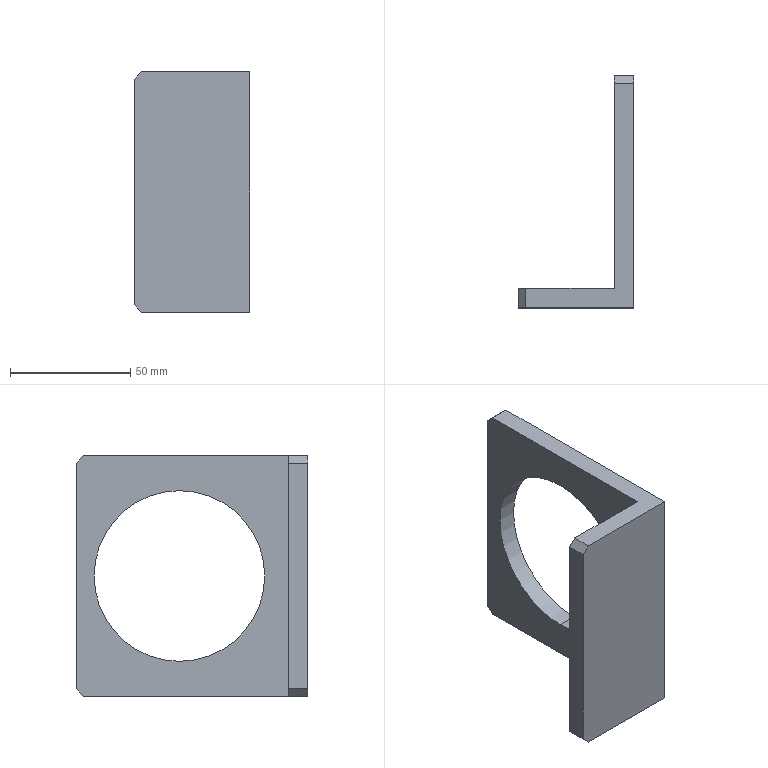Part | SolidWorks | features Chamfer 1, Extrusion 1, ICE 1 | 1 solid | 14 faces | box 48 x 96.5 x 100 mm | volume 77382 mm3 | plane 12 | cylinder 2 | commonest cylinder face diameters 71 x2
STEP:
#1=CARTESIAN_POINT('',(0.,53.5,1.121));
#2=VERTEX_POINT('',#1);
#3=CARTESIAN_POINT('',(0.,53.5,-69.879));
#4=VERTEX_POINT('',#3);
#5=CARTESIAN_POINT('',(0.,53.5,-34.379));
#6=DIRECTION('',(1.,0.,0.));
#7=DIRECTION('',(0.,0.,1.));
#8=AXIS2_PLACEMENT_3D('',#5,#6,#7);
#9=CIRCLE('',#8,35.5);
#10=EDGE_CURVE('',#2,#4,#9,.T.);
#11=ORIENTED_EDGE('',*,*,#10,.T.);
#12=CARTESIAN_POINT('',(-8.,53.5,-69.879));
#13=VERTEX_POINT('',#12);
#14=CARTESIAN_POINT('',(0.001,53.5,-69.879));
#15=DIRECTION('',(-1.,0.,0.));
#16=VECTOR('',#15,1000.);
#17=LINE('',#14,#16);
#18=EDGE_CURVE('',#4,#13,#17,.T.);
#19=ORIENTED_EDGE('',*,*,#18,.T.);
#20=CARTESIAN_POINT('',(-8.,53.5,1.121));
#21=VERTEX_POINT('',#20);
#22=CARTESIAN_POINT('',(-8.,53.5,-34.379));
#23=DIRECTION('',(-1.,0.,0.));
#24=DIRECTION('',(0.,0.,1.));
#25=AXIS2_PLACEMENT_3D('',#22,#23,#24);
#26=CIRCLE('',#25,35.5);
#27=EDGE_CURVE('',#13,#21,#26,.T.);
#28=ORIENTED_EDGE('',*,*,#27,.T.);
#29=CARTESIAN_POINT('',(0.001,53.5,1.121));
#30=DIRECTION('',(-1.,0.,0.));
#31=VECTOR('',#30,1000.);
#32=LINE('',#29,#31);
#33=EDGE_CURVE('',#2,#21,#32,.T.);
#34=ORIENTED_EDGE('',*,*,#33,.F.);
#35=EDGE_LOOP('',(#11,#19,#28,#34));
#36=FACE_OUTER_BOUND('',#35,.T.);
#37=CARTESIAN_POINT('',(0.001,53.5,-34.379));
#38=DIRECTION('',(-1.,0.,0.));
#39=DIRECTION('',(0.,0.,1.));
#40=AXIS2_PLACEMENT_3D('',#37,#38,#39);
#41=CYLINDRICAL_SURFACE('',#40,35.5);
#42=ADVANCED_FACE('',(#36),#41,.F.);
#43=CARTESIAN_POINT('',(-8.,96.5,12.621));
#44=VERTEX_POINT('',#43);
#45=CARTESIAN_POINT('',(-8.,96.5,-81.379));
#46=VERTEX_POINT('',#45);
#47=CARTESIAN_POINT('',(-8.,96.5,15.621));
#48=DIRECTION('',(0.,0.,-1.));
#49=VECTOR('',#48,1000.);
#50=LINE('',#47,#49);
#51=EDGE_CURVE('',#44,#46,#50,.T.);
#52=ORIENTED_EDGE('',*,*,#51,.F.);
#53=CARTESIAN_POINT('',(0.,96.5,12.621));
#54=VERTEX_POINT('',#53);
#55=CARTESIAN_POINT('',(-8.,96.5,12.621));
#56=DIRECTION('',(1.,0.,0.));
#57=VECTOR('',#56,1000.);
#58=LINE('',#55,#57);
#59=EDGE_CURVE('',#44,#54,#58,.T.);
#60=ORIENTED_EDGE('',*,*,#59,.T.);
#61=CARTESIAN_POINT('',(0.,96.5,-81.379));
#62=VERTEX_POINT('',#61);
#63=CARTESIAN_POINT('',(0.,96.5,15.621));
#64=DIRECTION('',(0.,0.,-1.));
#65=VECTOR('',#64,1000.);
#66=LINE('',#63,#65);
#67=EDGE_CURVE('',#54,#62,#66,.T.);
#68=ORIENTED_EDGE('',*,*,#67,.T.);
#69=CARTESIAN_POINT('',(-8.,96.5,-81.379));
#70=DIRECTION('',(-1.,0.,0.));
#71=VECTOR('',#70,1000.);
#72=LINE('',#69,#71);
#73=EDGE_CURVE('',#62,#46,#72,.T.);
#74=ORIENTED_EDGE('',*,*,#73,.T.);
#75=EDGE_LOOP('',(#52,#60,#68,#74));
#76=FACE_OUTER_BOUND('',#75,.T.);
#77=CARTESIAN_POINT('',(-8.,96.5,15.621));
#78=DIRECTION('',(0.,-1.,0.));
#79=DIRECTION('',(0.,0.,-1.));
#80=AXIS2_PLACEMENT_3D('',#77,#78,#79);
#81=PLANE('',#80);
#82=ADVANCED_FACE('',(#76),#81,.F.);
#83=CARTESIAN_POINT('',(-8.,53.5,-34.379));
#84=DIRECTION('',(-1.,0.,0.));
#85=DIRECTION('',(0.,0.,1.));
#86=AXIS2_PLACEMENT_3D('',#83,#84,#85);
#87=CIRCLE('',#86,35.5);
#88=EDGE_CURVE('',#21,#13,#87,.T.);
#89=ORIENTED_EDGE('',*,*,#88,.F.);
#90=ORIENTED_EDGE('',*,*,#27,.F.);
#91=EDGE_LOOP('',(#89,#90));
#92=FACE_BOUND('',#91,.T.);
#93=CARTESIAN_POINT('',(-8.,93.5,15.621));
#94=VERTEX_POINT('',#93);
#95=CARTESIAN_POINT('',(-8.,8.,15.621));
#96=VERTEX_POINT('',#95);
#97=CARTESIAN_POINT('',(-8.,8.,15.621));
#98=DIRECTION('',(0.,-1.,0.));
#99=VECTOR('',#98,1000.);
#100=LINE('',#97,#99);
#101=EDGE_CURVE('',#94,#96,#100,.T.);
#102=ORIENTED_EDGE('',*,*,#101,.F.);
#103=CARTESIAN_POINT('',(-8.,93.5,15.621));
#104=DIRECTION('',(0.,0.7071,-0.7071));
#105=VECTOR('',#104,1000.);
#106=LINE('',#103,#105);
#107=EDGE_CURVE('',#94,#44,#106,.T.);
#108=ORIENTED_EDGE('',*,*,#107,.T.);
#109=ORIENTED_EDGE('',*,*,#51,.T.);
#110=CARTESIAN_POINT('',(-8.,93.5,-84.379));
#111=VERTEX_POINT('',#110);
#112=CARTESIAN_POINT('',(-8.,96.5,-81.379));
#113=DIRECTION('',(0.,-0.7071,-0.7071));
#114=VECTOR('',#113,1000.);
#115=LINE('',#112,#114);
#116=EDGE_CURVE('',#46,#111,#115,.T.);
#117=ORIENTED_EDGE('',*,*,#116,.T.);
#118=CARTESIAN_POINT('',(-8.,8.,-84.379));
#119=VERTEX_POINT('',#118);
#120=CARTESIAN_POINT('',(-8.,8.,-84.379));
#121=DIRECTION('',(0.,-1.,0.));
#122=VECTOR('',#121,1000.);
#123=LINE('',#120,#122);
#124=EDGE_CURVE('',#111,#119,#123,.T.);
#125=ORIENTED_EDGE('',*,*,#124,.T.);
#126=CARTESIAN_POINT('',(-8.,8.,15.621));
#127=DIRECTION('',(0.,0.,-1.));
#128=VECTOR('',#127,1000.);
#129=LINE('',#126,#128);
#130=EDGE_CURVE('',#96,#119,#129,.T.);
#131=ORIENTED_EDGE('',*,*,#130,.F.);
#132=EDGE_LOOP('',(#102,#108,#109,#117,#125,#131));
#133=FACE_OUTER_BOUND('',#132,.T.);
#134=CARTESIAN_POINT('',(-8.,8.,15.621));
#135=DIRECTION('',(1.,0.,0.));
#136=DIRECTION('',(0.,0.,-1.));
#137=AXIS2_PLACEMENT_3D('',#134,#135,#136);
#138=PLANE('',#137);
#139=ADVANCED_FACE('',(#92,#133),#138,.F.);
#140=CARTESIAN_POINT('',(-45.,8.,-84.379));
#141=VERTEX_POINT('',#140);
#142=CARTESIAN_POINT('',(-48.,8.,-84.379));
#143=DIRECTION('',(-1.,0.,0.));
#144=VECTOR('',#143,1000.);
#145=LINE('',#142,#144);
#146=EDGE_CURVE('',#119,#141,#145,.T.);
#147=ORIENTED_EDGE('',*,*,#146,.T.);
#148=CARTESIAN_POINT('',(-48.,8.,-81.379));
#149=VERTEX_POINT('',#148);
#150=CARTESIAN_POINT('',(-48.,8.,-81.379));
#151=DIRECTION('',(-0.7071,0.,0.7071));
#152=VECTOR('',#151,1000.);
#153=LINE('',#150,#152);
#154=EDGE_CURVE('',#141,#149,#153,.T.);
#155=ORIENTED_EDGE('',*,*,#154,.T.);
#156=CARTESIAN_POINT('',(-48.,8.,12.621));
#157=VERTEX_POINT('',#156);
#158=CARTESIAN_POINT('',(-48.,8.,15.621));
#159=DIRECTION('',(0.,0.,-1.));
#160=VECTOR('',#159,1000.);
#161=LINE('',#158,#160);
#162=EDGE_CURVE('',#157,#149,#161,.T.);
#163=ORIENTED_EDGE('',*,*,#162,.F.);
#164=CARTESIAN_POINT('',(-45.,8.,15.621));
#165=VERTEX_POINT('',#164);
#166=CARTESIAN_POINT('',(-45.,8.,15.621));
#167=DIRECTION('',(0.7071,0.,0.7071));
#168=VECTOR('',#167,1000.);
#169=LINE('',#166,#168);
#170=EDGE_CURVE('',#157,#165,#169,.T.);
#171=ORIENTED_EDGE('',*,*,#170,.T.);
#172=CARTESIAN_POINT('',(-48.,8.,15.621));
#173=DIRECTION('',(-1.,0.,0.));
#174=VECTOR('',#173,1000.);
#175=LINE('',#172,#174);
#176=EDGE_CURVE('',#96,#165,#175,.T.);
#177=ORIENTED_EDGE('',*,*,#176,.F.);
#178=ORIENTED_EDGE('',*,*,#130,.T.);
#179=EDGE_LOOP('',(#147,#155,#163,#171,#177,#178));
#180=FACE_OUTER_BOUND('',#179,.T.);
#181=CARTESIAN_POINT('',(-48.,8.,15.621));
#182=DIRECTION('',(0.,-1.,0.));
#183=DIRECTION('',(1.,0.,0.));
#184=AXIS2_PLACEMENT_3D('',#181,#182,#183);
#185=PLANE('',#184);
#186=ADVANCED_FACE('',(#180),#185,.F.);
#187=ORIENTED_EDGE('',*,*,#162,.T.);
#188=CARTESIAN_POINT('',(-48.,0.,-81.379));
#189=VERTEX_POINT('',#188);
#190=CARTESIAN_POINT('',(-48.,0.,-81.379));
#191=DIRECTION('',(0.,-1.,0.));
#192=VECTOR('',#191,1000.);
#193=LINE('',#190,#192);
#194=EDGE_CURVE('',#149,#189,#193,.T.);
#195=ORIENTED_EDGE('',*,*,#194,.T.);
#196=CARTESIAN_POINT('',(-48.,0.,12.621));
#197=VERTEX_POINT('',#196);
#198=CARTESIAN_POINT('',(-48.,0.,15.621));
#199=DIRECTION('',(0.,0.,-1.));
#200=VECTOR('',#199,1000.);
#201=LINE('',#198,#200);
#202=EDGE_CURVE('',#197,#189,#201,.T.);
#203=ORIENTED_EDGE('',*,*,#202,.F.);
#204=CARTESIAN_POINT('',(-48.,0.,12.621));
#205=DIRECTION('',(0.,1.,0.));
#206=VECTOR('',#205,1000.);
#207=LINE('',#204,#206);
#208=EDGE_CURVE('',#197,#157,#207,.T.);
#209=ORIENTED_EDGE('',*,*,#208,.T.);
#210=EDGE_LOOP('',(#187,#195,#203,#209));
#211=FACE_OUTER_BOUND('',#210,.T.);
#212=CARTESIAN_POINT('',(-48.,0.,15.621));
#213=DIRECTION('',(1.,0.,0.));
#214=DIRECTION('',(0.,0.,-1.));
#215=AXIS2_PLACEMENT_3D('',#212,#213,#214);
#216=PLANE('',#215);
#217=ADVANCED_FACE('',(#211),#216,.F.);
#218=ORIENTED_EDGE('',*,*,#202,.T.);
#219=CARTESIAN_POINT('',(-45.,0.,-84.379));
#220=VERTEX_POINT('',#219);
#221=CARTESIAN_POINT('',(-48.,0.,-81.379));
#222=DIRECTION('',(0.7071,0.,-0.7071));
#223=VECTOR('',#222,1000.);
#224=LINE('',#221,#223);
#225=EDGE_CURVE('',#189,#220,#224,.T.);
#226=ORIENTED_EDGE('',*,*,#225,.T.);
#227=CARTESIAN_POINT('',(0.,0.,-84.379));
#228=VERTEX_POINT('',#227);
#229=CARTESIAN_POINT('',(0.,0.,-84.379));
#230=DIRECTION('',(1.,0.,0.));
#231=VECTOR('',#230,1000.);
#232=LINE('',#229,#231);
#233=EDGE_CURVE('',#220,#228,#232,.T.);
#234=ORIENTED_EDGE('',*,*,#233,.T.);
#235=CARTESIAN_POINT('',(0.,0.,15.621));
#236=VERTEX_POINT('',#235);
#237=CARTESIAN_POINT('',(0.,0.,15.621));
#238=DIRECTION('',(0.,0.,-1.));
#239=VECTOR('',#238,1000.);
#240=LINE('',#237,#239);
#241=EDGE_CURVE('',#236,#228,#240,.T.);
#242=ORIENTED_EDGE('',*,*,#241,.F.);
#243=CARTESIAN_POINT('',(-45.,0.,15.621));
#244=VERTEX_POINT('',#243);
#245=CARTESIAN_POINT('',(0.,0.,15.621));
#246=DIRECTION('',(1.,0.,0.));
#247=VECTOR('',#246,1000.);
#248=LINE('',#245,#247);
#249=EDGE_CURVE('',#244,#236,#248,.T.);
#250=ORIENTED_EDGE('',*,*,#249,.F.);
#251=CARTESIAN_POINT('',(-45.,0.,15.621));
#252=DIRECTION('',(-0.7071,0.,-0.7071));
#253=VECTOR('',#252,1000.);
#254=LINE('',#251,#253);
#255=EDGE_CURVE('',#244,#197,#254,.T.);
#256=ORIENTED_EDGE('',*,*,#255,.T.);
#257=EDGE_LOOP('',(#218,#226,#234,#242,#250,#256));
#258=FACE_OUTER_BOUND('',#257,.T.);
#259=CARTESIAN_POINT('',(0.,0.,15.621));
#260=DIRECTION('',(0.,1.,0.));
#261=DIRECTION('',(-1.,0.,0.));
#262=AXIS2_PLACEMENT_3D('',#259,#260,#261);
#263=PLANE('',#262);
#264=ADVANCED_FACE('',(#258),#263,.F.);
#265=ORIENTED_EDGE('',*,*,#10,.F.);
#266=CARTESIAN_POINT('',(0.,53.5,-34.379));
#267=DIRECTION('',(1.,0.,0.));
#268=DIRECTION('',(0.,0.,1.));
#269=AXIS2_PLACEMENT_3D('',#266,#267,#268);
#270=CIRCLE('',#269,35.5);
#271=EDGE_CURVE('',#4,#2,#270,.T.);
#272=ORIENTED_EDGE('',*,*,#271,.F.);
#273=EDGE_LOOP('',(#265,#272));
#274=FACE_BOUND('',#273,.T.);
#275=ORIENTED_EDGE('',*,*,#67,.F.);
#276=CARTESIAN_POINT('',(0.,93.5,15.621));
#277=VERTEX_POINT('',#276);
#278=CARTESIAN_POINT('',(0.,93.5,15.621));
#279=DIRECTION('',(0.,-0.7071,0.7071));
#280=VECTOR('',#279,1000.);
#281=LINE('',#278,#280);
#282=EDGE_CURVE('',#54,#277,#281,.T.);
#283=ORIENTED_EDGE('',*,*,#282,.T.);
#284=CARTESIAN_POINT('',(0.,96.5,15.621));
#285=DIRECTION('',(0.,1.,0.));
#286=VECTOR('',#285,1000.);
#287=LINE('',#284,#286);
#288=EDGE_CURVE('',#236,#277,#287,.T.);
#289=ORIENTED_EDGE('',*,*,#288,.F.);
#290=ORIENTED_EDGE('',*,*,#241,.T.);
#291=CARTESIAN_POINT('',(0.,93.5,-84.379));
#292=VERTEX_POINT('',#291);
#293=CARTESIAN_POINT('',(0.,96.5,-84.379));
#294=DIRECTION('',(0.,1.,0.));
#295=VECTOR('',#294,1000.);
#296=LINE('',#293,#295);
#297=EDGE_CURVE('',#228,#292,#296,.T.);
#298=ORIENTED_EDGE('',*,*,#297,.T.);
#299=CARTESIAN_POINT('',(0.,96.5,-81.379));
#300=DIRECTION('',(0.,0.7071,0.7071));
#301=VECTOR('',#300,1000.);
#302=LINE('',#299,#301);
#303=EDGE_CURVE('',#292,#62,#302,.T.);
#304=ORIENTED_EDGE('',*,*,#303,.T.);
#305=EDGE_LOOP('',(#275,#283,#289,#290,#298,#304));
#306=FACE_OUTER_BOUND('',#305,.T.);
#307=CARTESIAN_POINT('',(0.,96.5,15.621));
#308=DIRECTION('',(-1.,0.,0.));
#309=DIRECTION('',(0.,0.,1.));
#310=AXIS2_PLACEMENT_3D('',#307,#308,#309);
#311=PLANE('',#310);
#312=ADVANCED_FACE('',(#274,#306),#311,.F.);
#313=ORIENTED_EDGE('',*,*,#176,.T.);
#314=CARTESIAN_POINT('',(-45.,0.,15.621));
#315=DIRECTION('',(0.,-1.,0.));
#316=VECTOR('',#315,1000.);
#317=LINE('',#314,#316);
#318=EDGE_CURVE('',#165,#244,#317,.T.);
#319=ORIENTED_EDGE('',*,*,#318,.T.);
#320=ORIENTED_EDGE('',*,*,#249,.T.);
#321=ORIENTED_EDGE('',*,*,#288,.T.);
#322=CARTESIAN_POINT('',(0.,93.5,15.621));
#323=DIRECTION('',(-1.,0.,0.));
#324=VECTOR('',#323,1000.);
#325=LINE('',#322,#324);
#326=EDGE_CURVE('',#277,#94,#325,.T.);
#327=ORIENTED_EDGE('',*,*,#326,.T.);
#328=ORIENTED_EDGE('',*,*,#101,.T.);
#329=EDGE_LOOP('',(#313,#319,#320,#321,#327,#328));
#330=FACE_OUTER_BOUND('',#329,.T.);
#331=CARTESIAN_POINT('',(0.,0.,15.621));
#332=DIRECTION('',(0.,0.,-1.));
#333=DIRECTION('',(-1.,0.,0.));
#334=AXIS2_PLACEMENT_3D('',#331,#332,#333);
#335=PLANE('',#334);
#336=ADVANCED_FACE('',(#330),#335,.F.);
#337=ORIENTED_EDGE('',*,*,#233,.F.);
#338=CARTESIAN_POINT('',(-45.,8.,-84.379));
#339=DIRECTION('',(0.,1.,0.));
#340=VECTOR('',#339,1000.);
#341=LINE('',#338,#340);
#342=EDGE_CURVE('',#220,#141,#341,.T.);
#343=ORIENTED_EDGE('',*,*,#342,.T.);
#344=ORIENTED_EDGE('',*,*,#146,.F.);
#345=ORIENTED_EDGE('',*,*,#124,.F.);
#346=CARTESIAN_POINT('',(0.,93.5,-84.379));
#347=DIRECTION('',(1.,0.,0.));
#348=VECTOR('',#347,1000.);
#349=LINE('',#346,#348);
#350=EDGE_CURVE('',#111,#292,#349,.T.);
#351=ORIENTED_EDGE('',*,*,#350,.T.);
#352=ORIENTED_EDGE('',*,*,#297,.F.);
#353=EDGE_LOOP('',(#337,#343,#344,#345,#351,#352));
#354=FACE_OUTER_BOUND('',#353,.T.);
#355=CARTESIAN_POINT('',(0.,0.,-84.379));
#356=DIRECTION('',(0.,0.,-1.));
#357=DIRECTION('',(-1.,0.,0.));
#358=AXIS2_PLACEMENT_3D('',#355,#356,#357);
#359=PLANE('',#358);
#360=ADVANCED_FACE('',(#354),#359,.T.);
#361=ORIENTED_EDGE('',*,*,#154,.F.);
#362=ORIENTED_EDGE('',*,*,#342,.F.);
#363=ORIENTED_EDGE('',*,*,#225,.F.);
#364=ORIENTED_EDGE('',*,*,#194,.F.);
#365=EDGE_LOOP('',(#361,#362,#363,#364));
#366=FACE_OUTER_BOUND('',#365,.T.);
#367=CARTESIAN_POINT('',(-48.,0.,-81.379));
#368=DIRECTION('',(-0.7071,0.,-0.7071));
#369=DIRECTION('',(0.,1.,0.));
#370=AXIS2_PLACEMENT_3D('',#367,#368,#369);
#371=PLANE('',#370);
#372=ADVANCED_FACE('',(#366),#371,.T.);
#373=ORIENTED_EDGE('',*,*,#170,.F.);
#374=ORIENTED_EDGE('',*,*,#208,.F.);
#375=ORIENTED_EDGE('',*,*,#255,.F.);
#376=ORIENTED_EDGE('',*,*,#318,.F.);
#377=EDGE_LOOP('',(#373,#374,#375,#376));
#378=FACE_OUTER_BOUND('',#377,.T.);
#379=CARTESIAN_POINT('',(-45.,0.,15.621));
#380=DIRECTION('',(0.7071,0.,-0.7071));
#381=DIRECTION('',(0.,-1.,0.));
#382=AXIS2_PLACEMENT_3D('',#379,#380,#381);
#383=PLANE('',#382);
#384=ADVANCED_FACE('',(#378),#383,.F.);
#385=ORIENTED_EDGE('',*,*,#282,.F.);
#386=ORIENTED_EDGE('',*,*,#59,.F.);
#387=ORIENTED_EDGE('',*,*,#107,.F.);
#388=ORIENTED_EDGE('',*,*,#326,.F.);
#389=EDGE_LOOP('',(#385,#386,#387,#388));
#390=FACE_OUTER_BOUND('',#389,.T.);
#391=CARTESIAN_POINT('',(0.,93.5,15.621));
#392=DIRECTION('',(0.,-0.7071,-0.7071));
#393=DIRECTION('',(-1.,0.,0.));
#394=AXIS2_PLACEMENT_3D('',#391,#392,#393);
#395=PLANE('',#394);
#396=ADVANCED_FACE('',(#390),#395,.F.);
#397=ORIENTED_EDGE('',*,*,#303,.F.);
#398=ORIENTED_EDGE('',*,*,#350,.F.);
#399=ORIENTED_EDGE('',*,*,#116,.F.);
#400=ORIENTED_EDGE('',*,*,#73,.F.);
#401=EDGE_LOOP('',(#397,#398,#399,#400));
#402=FACE_OUTER_BOUND('',#401,.T.);
#403=CARTESIAN_POINT('',(-8.,96.5,-81.379));
#404=DIRECTION('',(0.,0.7071,-0.7071));
#405=DIRECTION('',(1.,0.,0.));
#406=AXIS2_PLACEMENT_3D('',#403,#404,#405);
#407=PLANE('',#406);
#408=ADVANCED_FACE('',(#402),#407,.T.);
#409=ORIENTED_EDGE('',*,*,#18,.F.);
#410=ORIENTED_EDGE('',*,*,#271,.T.);
#411=ORIENTED_EDGE('',*,*,#33,.T.);
#412=ORIENTED_EDGE('',*,*,#88,.T.);
#413=EDGE_LOOP('',(#409,#410,#411,#412));
#414=FACE_OUTER_BOUND('',#413,.T.);
#415=CARTESIAN_POINT('',(0.001,53.5,-34.379));
#416=DIRECTION('',(-1.,0.,0.));
#417=DIRECTION('',(0.,0.,1.));
#418=AXIS2_PLACEMENT_3D('',#415,#416,#417);
#419=CYLINDRICAL_SURFACE('',#418,35.5);
#420=ADVANCED_FACE('',(#414),#419,.F.);
#421=CLOSED_SHELL('',(#42,#82,#139,#186,#217,#264,#312,#336,#360,#372,#384,#396,#408,#420));
#422=MANIFOLD_SOLID_BREP('',#421);
#423=CARTESIAN_POINT('',(0.,0.,0.));
#424=DIRECTION('',(0.,0.,1.));
#425=DIRECTION('',(1.,0.,0.));
#426=AXIS2_PLACEMENT_3D('',#423,#424,#425);
#427=(LENGTH_UNIT()NAMED_UNIT(*)SI_UNIT(.MILLI.,.METRE.));
#428=UNCERTAINTY_MEASURE_WITH_UNIT(LENGTH_MEASURE(0.00001),#427,'','');
#429=(NAMED_UNIT(*)PLANE_ANGLE_UNIT()SI_UNIT($,.RADIAN.));
#430=(NAMED_UNIT(*)SI_UNIT($,.STERADIAN.)SOLID_ANGLE_UNIT());
#431=(GEOMETRIC_REPRESENTATION_CONTEXT(3)GLOBAL_UNCERTAINTY_ASSIGNED_CONTEXT((#428))GLOBAL_UNIT_ASSIGNED_CONTEXT((#427,#429,#430))REPRESENTATION_CONTEXT('',''));
#432=ADVANCED_BREP_SHAPE_REPRESENTATION('',(#422,#426),#431);